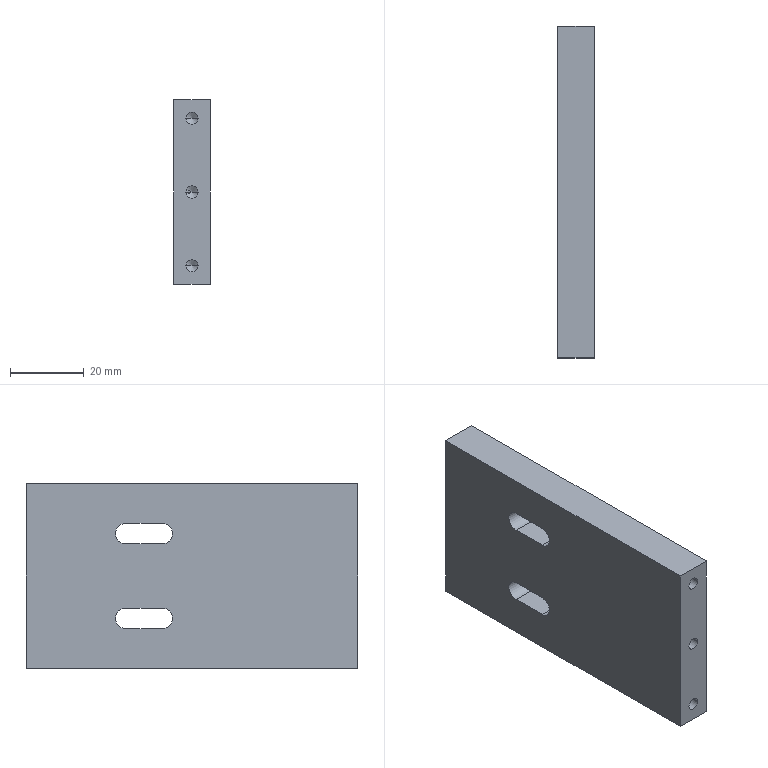Part | STEP file | 04-16 Heat-shrink press cylinder fixing plate | 1 solid | 26 faces | box 10 x 90 x 50 mm | volume 43055 mm3 | cylinder 10 | plane 10 | cone 6 | commonest cylinder face diameters 3.3 x6 5.5 x4